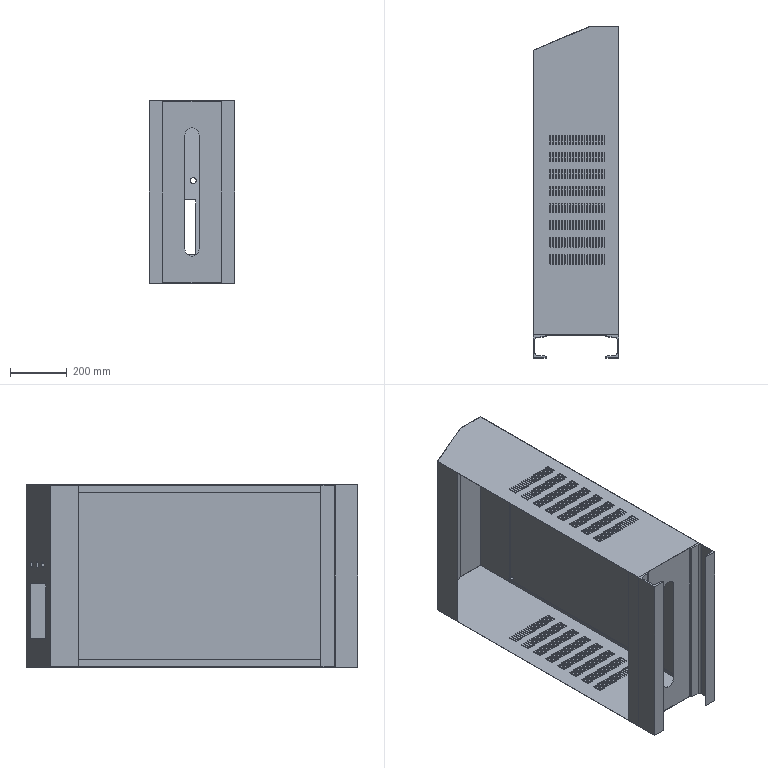Part | STEP file | PN_0027 | 3 solids | 1398 faces | box 300 x 1165 x 640 mm | volume 4220898 mm3 | plane 726 | cylinder 672 | commonest cylinder face diameters 3 x640 8 x12 9 x8 22 x6 16 x4 50 x2